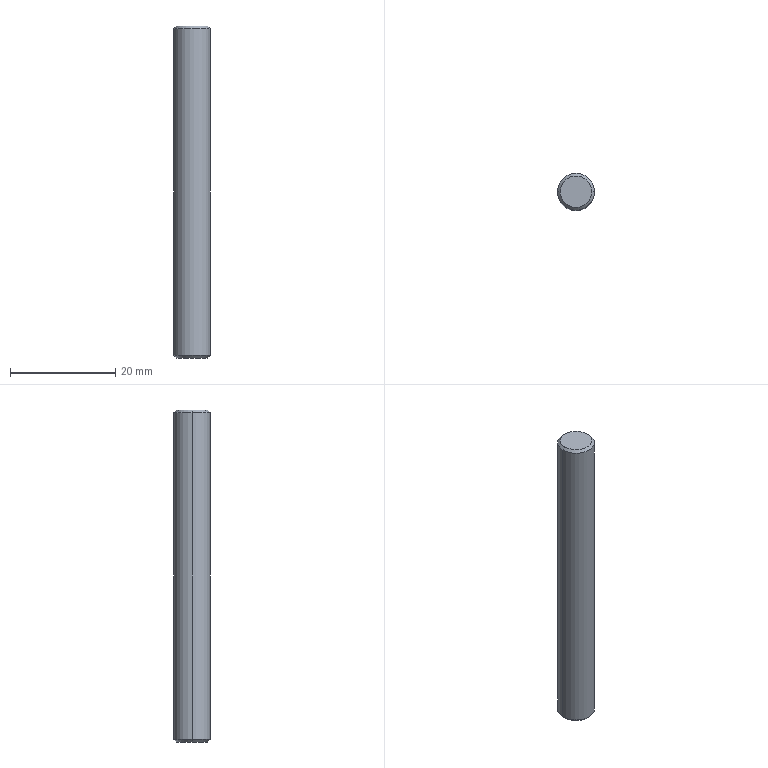Part | STEP file | _AKQ01怡合达销1 | 1 solid | 8 faces | box 7 x 7 x 63 mm | volume 2419 mm3 | cone 4 | cylinder 2 | plane 2 | commonest cylinder face diameters 7 x2
STEP:
#1=CARTESIAN_POINT('',(3.,0.,31.5));
#2=VERTEX_POINT('',#1);
#3=CARTESIAN_POINT('',(-3.,0.,31.5));
#4=VERTEX_POINT('',#3);
#5=CARTESIAN_POINT('',(0.,0.,31.5));
#6=DIRECTION('',(0.,0.,1.));
#7=DIRECTION('',(1.,0.,0.));
#8=AXIS2_PLACEMENT_3D('',#5,#6,#7);
#9=CIRCLE('',#8,3.);
#10=EDGE_CURVE('',#2,#4,#9,.T.);
#11=ORIENTED_EDGE('',*,*,#10,.F.);
#12=CARTESIAN_POINT('',(3.5,0.,31.));
#13=VERTEX_POINT('',#12);
#14=CARTESIAN_POINT('',(3.,0.,31.5));
#15=DIRECTION('',(0.7071,0.,-0.7071));
#16=VECTOR('',#15,1000.);
#17=LINE('',#14,#16);
#18=EDGE_CURVE('',#2,#13,#17,.T.);
#19=ORIENTED_EDGE('',*,*,#18,.T.);
#20=CARTESIAN_POINT('',(-3.5,0.,31.));
#21=VERTEX_POINT('',#20);
#22=CARTESIAN_POINT('',(0.,0.,31.));
#23=DIRECTION('',(0.,0.,-1.));
#24=DIRECTION('',(1.,0.,0.));
#25=AXIS2_PLACEMENT_3D('',#22,#23,#24);
#26=CIRCLE('',#25,3.5);
#27=EDGE_CURVE('',#21,#13,#26,.T.);
#28=ORIENTED_EDGE('',*,*,#27,.F.);
#29=CARTESIAN_POINT('',(-3.,0.,31.5));
#30=DIRECTION('',(-0.7071,0.,-0.7071));
#31=VECTOR('',#30,1000.);
#32=LINE('',#29,#31);
#33=EDGE_CURVE('',#4,#21,#32,.T.);
#34=ORIENTED_EDGE('',*,*,#33,.F.);
#35=EDGE_LOOP('',(#11,#19,#28,#34));
#36=FACE_OUTER_BOUND('',#35,.T.);
#37=CARTESIAN_POINT('',(0.,0.,31.5));
#38=DIRECTION('',(0.,0.,-1.));
#39=DIRECTION('',(-1.,0.,0.));
#40=AXIS2_PLACEMENT_3D('',#37,#38,#39);
#41=CONICAL_SURFACE('',#40,3.,0.7854);
#42=ADVANCED_FACE('',(#36),#41,.T.);
#43=CARTESIAN_POINT('',(-3.,0.,-31.5));
#44=VERTEX_POINT('',#43);
#45=CARTESIAN_POINT('',(3.,0.,-31.5));
#46=VERTEX_POINT('',#45);
#47=CARTESIAN_POINT('',(0.,0.,-31.5));
#48=DIRECTION('',(0.,0.,-1.));
#49=DIRECTION('',(1.,0.,0.));
#50=AXIS2_PLACEMENT_3D('',#47,#48,#49);
#51=CIRCLE('',#50,3.);
#52=EDGE_CURVE('',#44,#46,#51,.T.);
#53=ORIENTED_EDGE('',*,*,#52,.F.);
#54=CARTESIAN_POINT('',(-3.5,0.,-31.));
#55=VERTEX_POINT('',#54);
#56=CARTESIAN_POINT('',(-3.5,0.,-31.));
#57=DIRECTION('',(-0.7071,0.,0.7071));
#58=VECTOR('',#57,1000.);
#59=LINE('',#56,#58);
#60=EDGE_CURVE('',#44,#55,#59,.T.);
#61=ORIENTED_EDGE('',*,*,#60,.T.);
#62=CARTESIAN_POINT('',(3.5,0.,-31.));
#63=VERTEX_POINT('',#62);
#64=CARTESIAN_POINT('',(0.,0.,-31.));
#65=DIRECTION('',(0.,0.,1.));
#66=DIRECTION('',(1.,0.,0.));
#67=AXIS2_PLACEMENT_3D('',#64,#65,#66);
#68=CIRCLE('',#67,3.5);
#69=EDGE_CURVE('',#63,#55,#68,.T.);
#70=ORIENTED_EDGE('',*,*,#69,.F.);
#71=CARTESIAN_POINT('',(3.5,0.,-31.));
#72=DIRECTION('',(0.7071,0.,0.7071));
#73=VECTOR('',#72,1000.);
#74=LINE('',#71,#73);
#75=EDGE_CURVE('',#46,#63,#74,.T.);
#76=ORIENTED_EDGE('',*,*,#75,.F.);
#77=EDGE_LOOP('',(#53,#61,#70,#76));
#78=FACE_OUTER_BOUND('',#77,.T.);
#79=CARTESIAN_POINT('',(0.,0.,-31.));
#80=DIRECTION('',(0.,0.,1.));
#81=DIRECTION('',(1.,0.,0.));
#82=AXIS2_PLACEMENT_3D('',#79,#80,#81);
#83=CONICAL_SURFACE('',#82,3.5,0.7854);
#84=ADVANCED_FACE('',(#78),#83,.T.);
#85=ORIENTED_EDGE('',*,*,#27,.T.);
#86=CARTESIAN_POINT('',(3.5,0.,31.5));
#87=DIRECTION('',(0.,0.,-1.));
#88=VECTOR('',#87,1000.);
#89=LINE('',#86,#88);
#90=EDGE_CURVE('',#13,#63,#89,.T.);
#91=ORIENTED_EDGE('',*,*,#90,.T.);
#92=ORIENTED_EDGE('',*,*,#69,.T.);
#93=CARTESIAN_POINT('',(-3.5,0.,31.5));
#94=DIRECTION('',(0.,0.,-1.));
#95=VECTOR('',#94,1000.);
#96=LINE('',#93,#95);
#97=EDGE_CURVE('',#21,#55,#96,.T.);
#98=ORIENTED_EDGE('',*,*,#97,.F.);
#99=EDGE_LOOP('',(#85,#91,#92,#98));
#100=FACE_OUTER_BOUND('',#99,.T.);
#101=CARTESIAN_POINT('',(0.,0.,31.5));
#102=DIRECTION('',(0.,0.,-1.));
#103=DIRECTION('',(-1.,0.,0.));
#104=AXIS2_PLACEMENT_3D('',#101,#102,#103);
#105=CYLINDRICAL_SURFACE('',#104,3.5);
#106=ADVANCED_FACE('',(#100),#105,.T.);
#107=ORIENTED_EDGE('',*,*,#90,.F.);
#108=CARTESIAN_POINT('',(0.,0.,31.));
#109=DIRECTION('',(0.,0.,-1.));
#110=DIRECTION('',(1.,0.,0.));
#111=AXIS2_PLACEMENT_3D('',#108,#109,#110);
#112=CIRCLE('',#111,3.5);
#113=EDGE_CURVE('',#13,#21,#112,.T.);
#114=ORIENTED_EDGE('',*,*,#113,.T.);
#115=ORIENTED_EDGE('',*,*,#97,.T.);
#116=CARTESIAN_POINT('',(0.,0.,-31.));
#117=DIRECTION('',(0.,0.,1.));
#118=DIRECTION('',(1.,0.,0.));
#119=AXIS2_PLACEMENT_3D('',#116,#117,#118);
#120=CIRCLE('',#119,3.5);
#121=EDGE_CURVE('',#55,#63,#120,.T.);
#122=ORIENTED_EDGE('',*,*,#121,.T.);
#123=EDGE_LOOP('',(#107,#114,#115,#122));
#124=FACE_OUTER_BOUND('',#123,.T.);
#125=CARTESIAN_POINT('',(0.,0.,31.5));
#126=DIRECTION('',(0.,0.,-1.));
#127=DIRECTION('',(-1.,0.,0.));
#128=AXIS2_PLACEMENT_3D('',#125,#126,#127);
#129=CYLINDRICAL_SURFACE('',#128,3.5);
#130=ADVANCED_FACE('',(#124),#129,.T.);
#131=CARTESIAN_POINT('',(0.,0.,31.5));
#132=DIRECTION('',(0.,0.,1.));
#133=DIRECTION('',(1.,0.,0.));
#134=AXIS2_PLACEMENT_3D('',#131,#132,#133);
#135=CIRCLE('',#134,3.);
#136=EDGE_CURVE('',#4,#2,#135,.T.);
#137=ORIENTED_EDGE('',*,*,#136,.T.);
#138=ORIENTED_EDGE('',*,*,#10,.T.);
#139=EDGE_LOOP('',(#137,#138));
#140=FACE_OUTER_BOUND('',#139,.T.);
#141=CARTESIAN_POINT('',(0.,0.,31.5));
#142=DIRECTION('',(0.,0.,1.));
#143=DIRECTION('',(1.,0.,0.));
#144=AXIS2_PLACEMENT_3D('',#141,#142,#143);
#145=PLANE('',#144);
#146=ADVANCED_FACE('',(#140),#145,.T.);
#147=CARTESIAN_POINT('',(0.,0.,-31.5));
#148=DIRECTION('',(0.,0.,-1.));
#149=DIRECTION('',(1.,0.,0.));
#150=AXIS2_PLACEMENT_3D('',#147,#148,#149);
#151=CIRCLE('',#150,3.);
#152=EDGE_CURVE('',#46,#44,#151,.T.);
#153=ORIENTED_EDGE('',*,*,#152,.T.);
#154=ORIENTED_EDGE('',*,*,#52,.T.);
#155=EDGE_LOOP('',(#153,#154));
#156=FACE_OUTER_BOUND('',#155,.T.);
#157=CARTESIAN_POINT('',(0.,0.,-31.5));
#158=DIRECTION('',(0.,0.,1.));
#159=DIRECTION('',(1.,0.,0.));
#160=AXIS2_PLACEMENT_3D('',#157,#158,#159);
#161=PLANE('',#160);
#162=ADVANCED_FACE('',(#156),#161,.F.);
#163=ORIENTED_EDGE('',*,*,#60,.F.);
#164=ORIENTED_EDGE('',*,*,#152,.F.);
#165=ORIENTED_EDGE('',*,*,#75,.T.);
#166=ORIENTED_EDGE('',*,*,#121,.F.);
#167=EDGE_LOOP('',(#163,#164,#165,#166));
#168=FACE_OUTER_BOUND('',#167,.T.);
#169=CARTESIAN_POINT('',(0.,0.,-31.));
#170=DIRECTION('',(0.,0.,1.));
#171=DIRECTION('',(1.,0.,0.));
#172=AXIS2_PLACEMENT_3D('',#169,#170,#171);
#173=CONICAL_SURFACE('',#172,3.5,0.7854);
#174=ADVANCED_FACE('',(#168),#173,.T.);
#175=ORIENTED_EDGE('',*,*,#18,.F.);
#176=ORIENTED_EDGE('',*,*,#136,.F.);
#177=ORIENTED_EDGE('',*,*,#33,.T.);
#178=ORIENTED_EDGE('',*,*,#113,.F.);
#179=EDGE_LOOP('',(#175,#176,#177,#178));
#180=FACE_OUTER_BOUND('',#179,.T.);
#181=CARTESIAN_POINT('',(0.,0.,31.5));
#182=DIRECTION('',(0.,0.,-1.));
#183=DIRECTION('',(-1.,0.,0.));
#184=AXIS2_PLACEMENT_3D('',#181,#182,#183);
#185=CONICAL_SURFACE('',#184,3.,0.7854);
#186=ADVANCED_FACE('',(#180),#185,.T.);
#187=CLOSED_SHELL('',(#42,#84,#106,#130,#146,#162,#174,#186));
#188=MANIFOLD_SOLID_BREP('',#187);
#189=CARTESIAN_POINT('',(0.,0.,0.));
#190=DIRECTION('',(0.,0.,1.));
#191=DIRECTION('',(1.,0.,0.));
#192=AXIS2_PLACEMENT_3D('',#189,#190,#191);
#193=(LENGTH_UNIT()NAMED_UNIT(*)SI_UNIT(.MILLI.,.METRE.));
#194=UNCERTAINTY_MEASURE_WITH_UNIT(LENGTH_MEASURE(0.00001),#193,'','');
#195=(NAMED_UNIT(*)PLANE_ANGLE_UNIT()SI_UNIT($,.RADIAN.));
#196=(NAMED_UNIT(*)SI_UNIT($,.STERADIAN.)SOLID_ANGLE_UNIT());
#197=(GEOMETRIC_REPRESENTATION_CONTEXT(3)GLOBAL_UNCERTAINTY_ASSIGNED_CONTEXT((#194))GLOBAL_UNIT_ASSIGNED_CONTEXT((#193,#195,#196))REPRESENTATION_CONTEXT('',''));
#198=ADVANCED_BREP_SHAPE_REPRESENTATION('',(#188,#192),#197);